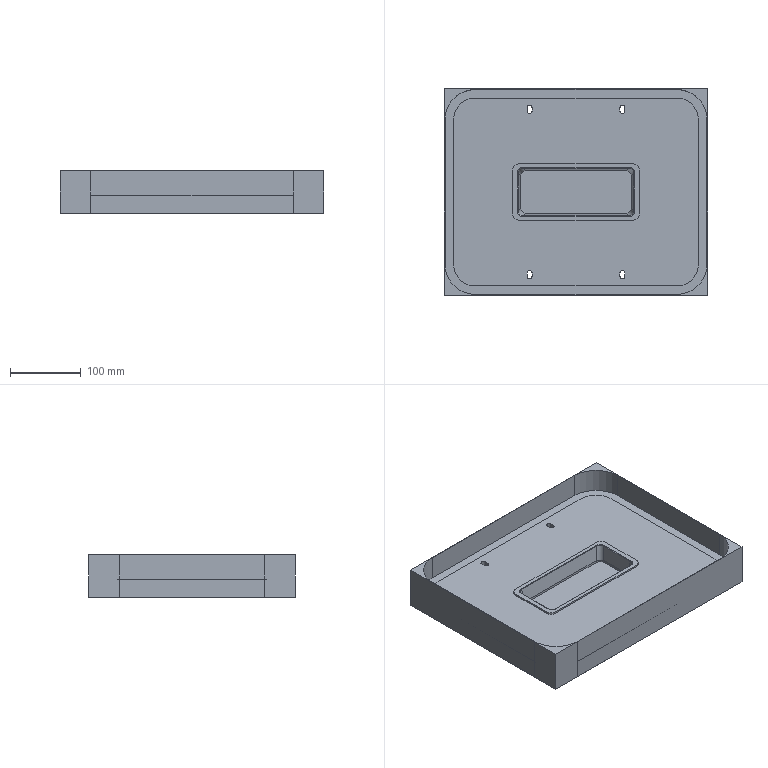NC program | NX | posted with a generic post | part box 371 x 291 x 60.5 mm
Lines 1 to 1445 of 37416:
N10 G17 G21 G94 G90
(CAVITY_MILL , TOOL : D16R0.8)
N12 T00 M6
N14 G53
N16 G17 G0 G90 X-26.999 Y136.323 S8000 M3 M8
N18 G43 Z120.5 H0
N20 Z61.5
N22 G94 G1 X0. Z60.085 F4500.
N24 X142.5
N26 G2 X176.323 Y102.5 R33.823
N28 G1 Y-102.506
N30 G2 X142.5 Y-136.323 R33.823
N32 G1 X-142.5
N34 G2 X-176.323 Y-102.5 R33.823
N36 G1 Y102.5
N38 G2 X-142.5 Y136.323 R33.823
N40 G1 X0.
N42 Y126.243
N44 X142.5
N46 G2 X166.243 Y102.5 R23.743
N48 G1 Y-102.504
N50 G2 X142.5 Y-126.243 R23.743
N52 G1 X-142.5
N54 G2 X-166.243 Y-102.5 R23.743
N56 G1 Y102.5
N58 G2 X-142.5 Y126.243 R23.743
N60 G1 X0.
N62 Y116.163
N64 X142.5
N66 G2 X156.163 Y102.5 R13.663
N68 G1 Y-102.504
N70 G2 X142.5 Y-116.163 R13.663
N72 G1 X-142.5
N74 G2 X-156.163 Y-102.5 R13.663
N76 G1 Y102.5
N78 G2 X-142.5 Y116.163 R13.663
N80 G1 X0.
N82 Y106.083
N84 X142.5
N86 G2 X146.083 Y102.5 R3.583
N88 G1 Y-102.502
N90 G2 X142.5 Y-106.083 R3.583
N92 G1 X-142.5
N94 G2 X-146.083 Y-102.5 R3.583
N96 G1 Y102.5
N98 G2 X-142.5 Y106.083 R3.583
N100 G1 X0.
N102 Y96.003
N104 X136.003
N106 Y-96.003
N108 X-136.003
N110 Y96.003
N112 X0.
N114 Y85.923
N116 X125.923
N118 Y-85.923
N120 X-125.923
N122 Y85.923
N124 X0.
N126 Y75.843
N128 X115.843
N130 Y-75.843
N132 X-115.843
N134 Y75.843
N136 X0.
N138 Y65.763
N140 X105.763
N142 Y-65.763
N144 X-105.763
N146 Y65.763
N148 X0.
N150 Y55.683
N152 X95.683
N154 Y-55.683
N156 X-95.683
N158 Y55.683
N160 X0.
N162 Y45.603
N164 X85.603
N166 Y-45.603
N168 X-85.603
N170 Y45.603
N172 X0.
N174 Y35.523
N176 X75.523
N178 Y-35.523
N180 X-75.523
N182 Y35.523
N184 X0.
N186 Y25.443
N188 X65.443
N190 Y-25.443
N192 X-65.443
N194 Y25.443
N196 X0.
N198 Y15.363
N200 X55.363
N202 Y-15.363
N204 X-55.363
N206 Y15.363
N208 X0.
N210 Y5.283
N212 X45.283
N214 Y-5.283
N216 X-45.283
N218 Y5.283
N220 X0.
N222 G3 X3.2 Y8.483 R3.2
N224 G1 Z61.085
N226 G0 Z63.5
N228 X-26.999 Y136.25
N230 Z61.085
N232 G1 X0. Z59.67
N234 X142.5
N236 G2 X176.25 Y102.506 R33.75
N238 G1 Y-102.506
N240 G2 X142.5 Y-136.25 R33.75
N242 G1 X-142.5
N244 G2 X-176.25 Y-102.5 R33.75
N246 G1 Y102.5
N248 G2 X-142.5 Y136.25 R33.75
N250 G1 X0.
N252 Y126.17
N254 X142.5
N256 G2 X166.17 Y102.504 R23.67
N258 G1 Y-102.504
N260 G2 X142.5 Y-126.17 R23.67
N262 G1 X-142.5
N264 G2 X-166.17 Y-102.5 R23.67
N266 G1 Y102.5
N268 G2 X-142.5 Y126.17 R23.67
N270 G1 X0.
N272 Y116.09
N274 X142.5
N276 G2 X156.09 Y102.502 R13.59
N278 G1 Y-102.504
N280 G2 X142.5 Y-116.09 R13.59
N282 G1 X-142.5
N284 G2 X-156.09 Y-102.5 R13.59
N286 G1 Y102.5
N288 G2 X-142.5 Y116.09 R13.59
N290 G1 X0.
N292 Y106.01
N294 X142.5
N296 G2 X146.01 Y102.501 R3.51
N298 G1 Y-102.502
N300 G2 X142.5 Y-106.01 R3.51
N302 G1 X-142.5
N304 G2 X-146.01 Y-102.5 R3.51
N306 G1 Y102.5
N308 G2 X-142.5 Y106.01 R3.51
N310 G1 X0.
N312 Y95.93
N314 X135.93
N316 Y-95.93
N318 X-135.93
N320 Y95.93
N322 X0.
N324 Y85.85
N326 X125.85
N328 Y-85.85
N330 X-125.85
N332 Y85.85
N334 X0.
N336 Y75.77
N338 X115.77
N340 Y-75.77
N342 X-115.77
N344 Y75.77
N346 X0.
N348 Y65.69
N350 X105.69
N352 Y-65.69
N354 X-105.69
N356 Y65.69
N358 X0.
N360 Y55.61
N362 X95.61
N364 Y-55.61
N366 X-95.61
N368 Y55.61
N370 X0.
N372 Y45.53
N374 X85.53
N376 Y-45.53
N378 X-85.53
N380 Y45.53
N382 X0.
N384 Y35.45
N386 X75.45
N388 Y-35.45
N390 X-75.45
N392 Y35.45
N394 X0.
N396 Y25.37
N398 X65.37
N400 Y-25.37
N402 X-65.37
N404 Y25.37
N406 X0.
N408 Y15.29
N410 X55.29
N412 Y-15.29
N414 X-55.29
N416 Y15.29
N418 X0.
N420 Y5.21
N422 X45.21
N424 Y-5.21
N426 X-45.21
N428 Y5.21
N430 X0.
N432 G3 X3.2 Y8.41 R3.2
N434 G1 Z60.67
N436 G0 Z63.085
N438 X-26.999 Y136.25
N440 Z60.67
N442 G1 X0. Z59.255
N444 X142.5
N446 G2 X176.25 Y102.506 R33.75
N448 G1 Y-102.506
N450 G2 X142.5 Y-136.25 R33.75
N452 G1 X-142.5
N454 G2 X-176.25 Y-102.5 R33.75
N456 G1 Y102.5
N458 G2 X-142.5 Y136.25 R33.75
N460 G1 X0.
N462 Y126.17
N464 X142.5
N466 G2 X166.17 Y102.504 R23.67
N468 G1 Y-102.504
N470 G2 X142.5 Y-126.17 R23.67
N472 G1 X-142.5
N474 G2 X-166.17 Y-102.5 R23.67
N476 G1 Y102.5
N478 G2 X-142.5 Y126.17 R23.67
N480 G1 X0.
N482 Y116.09
N484 X142.5
N486 G2 X156.09 Y102.502 R13.59
N488 G1 Y-102.504
N490 G2 X142.5 Y-116.09 R13.59
N492 G1 X-142.5
N494 G2 X-156.09 Y-102.5 R13.59
N496 G1 Y102.5
N498 G2 X-142.5 Y116.09 R13.59
N500 G1 X0.
N502 Y106.01
N504 X142.5
N506 G2 X146.01 Y102.501 R3.51
N508 G1 Y-102.502
N510 G2 X142.5 Y-106.01 R3.51
N512 G1 X-142.5
N514 G2 X-146.01 Y-102.5 R3.51
N516 G1 Y102.5
N518 G2 X-142.5 Y106.01 R3.51
N520 G1 X0.
N522 Y95.93
N524 X135.93
N526 Y-95.93
N528 X-135.93
N530 Y95.93
N532 X0.
N534 Y85.85
N536 X125.85
N538 Y-85.85
N540 X-125.85
N542 Y85.85
N544 X0.
N546 Y75.77
N548 X115.77
N550 Y-75.77
N552 X-115.77
N554 Y75.77
N556 X0.
N558 Y65.69
N560 X105.69
N562 Y-65.69
N564 X-105.69
N566 Y65.69
N568 X0.
N570 Y55.61
N572 X95.61
N574 Y-55.61
N576 X-95.61
N578 Y55.61
N580 X0.
N582 Y45.53
N584 X85.53
N586 Y-45.53
N588 X-85.53
N590 Y45.53
N592 X0.
N594 Y35.45
N596 X75.45
N598 Y-35.45
N600 X-75.45
N602 Y35.45
N604 X0.
N606 Y25.37
N608 X65.37
N610 Y-25.37
N612 X-65.37
N614 Y25.37
N616 X0.
N618 Y15.29
N620 X55.29
N622 Y-15.29
N624 X-55.29
N626 Y15.29
N628 X0.
N630 Y5.21
N632 X45.21
N634 Y-5.21
N636 X-45.21
N638 Y5.21
N640 X0.
N642 G3 X3.2 Y8.41 R3.2
N644 G1 Z60.255
N646 G0 Z62.67
N648 X-26.999 Y136.25
N650 Z60.255
N652 G1 X0. Z58.84
N654 X142.5
N656 G2 X176.25 Y102.506 R33.75
N658 G1 Y-102.506
N660 G2 X142.5 Y-136.25 R33.75
N662 G1 X-142.5
N664 G2 X-176.25 Y-102.5 R33.75
N666 G1 Y102.5
N668 G2 X-142.5 Y136.25 R33.75
N670 G1 X0.
N672 Y126.17
N674 X142.5
N676 G2 X166.17 Y102.504 R23.67
N678 G1 Y-102.504
N680 G2 X142.5 Y-126.17 R23.67
N682 G1 X-142.5
N684 G2 X-166.17 Y-102.5 R23.67
N686 G1 Y102.5
N688 G2 X-142.5 Y126.17 R23.67
N690 G1 X0.
N692 Y116.09
N694 X142.5
N696 G2 X156.09 Y102.502 R13.59
N698 G1 Y-102.504
N700 G2 X142.5 Y-116.09 R13.59
N702 G1 X-142.5
N704 G2 X-156.09 Y-102.5 R13.59
N706 G1 Y102.5
N708 G2 X-142.5 Y116.09 R13.59
N710 G1 X0.
N712 Y106.01
N714 X142.5
N716 G2 X146.01 Y102.501 R3.51
N718 G1 Y-102.502
N720 G2 X142.5 Y-106.01 R3.51
N722 G1 X-142.5
N724 G2 X-146.01 Y-102.5 R3.51
N726 G1 Y102.5
N728 G2 X-142.5 Y106.01 R3.51
N730 G1 X0.
N732 Y95.93
N734 X135.93
N736 Y-95.93
N738 X-135.93
N740 Y95.93
N742 X0.
N744 Y85.85
N746 X125.85
N748 Y-85.85
N750 X-125.85
N752 Y85.85
N754 X0.
N756 Y75.77
N758 X115.77
N760 Y-75.77
N762 X-115.77
N764 Y75.77
N766 X0.
N768 Y65.69
N770 X105.69
N772 Y-65.69
N774 X-105.69
N776 Y65.69
N778 X0.
N780 Y55.61
N782 X95.61
N784 Y-55.61
N786 X-95.61
N788 Y55.61
N790 X0.
N792 Y45.53
N794 X85.53
N796 Y-45.53
N798 X-85.53
N800 Y45.53
N802 X0.
N804 Y35.45
N806 X75.45
N808 Y-35.45
N810 X-75.45
N812 Y35.45
N814 X0.
N816 Y25.37
N818 X65.37
N820 Y-25.37
N822 X-65.37
N824 Y25.37
N826 X0.
N828 Y15.29
N830 X55.29
N832 Y-15.29
N834 X-55.29
N836 Y15.29
N838 X0.
N840 Y5.21
N842 X45.21
N844 Y-5.21
N846 X-45.21
N848 Y5.21
N850 X0.
N852 G3 X3.2 Y8.41 R3.2
N854 G1 Z59.84
N856 G0 Z62.255
N858 X-26.999 Y136.25
N860 Z59.84
N862 G1 X0. Z58.425
N864 X142.5
N866 G2 X176.25 Y102.506 R33.75
N868 G1 Y-102.506
N870 G2 X142.5 Y-136.25 R33.75
N872 G1 X-142.5
N874 G2 X-176.25 Y-102.5 R33.75
N876 G1 Y102.5
N878 G2 X-142.5 Y136.25 R33.75
N880 G1 X0.
N882 Y126.17
N884 X142.5
N886 G2 X166.17 Y102.504 R23.67
N888 G1 Y-102.504
N890 G2 X142.5 Y-126.17 R23.67
N892 G1 X-142.5
N894 G2 X-166.17 Y-102.5 R23.67
N896 G1 Y102.5
N898 G2 X-142.5 Y126.17 R23.67
N900 G1 X0.
N902 Y116.09
N904 X142.5
N906 G2 X156.09 Y102.502 R13.59
N908 G1 Y-102.504
N910 G2 X142.5 Y-116.09 R13.59
N912 G1 X-142.5
N914 G2 X-156.09 Y-102.5 R13.59
N916 G1 Y102.5
N918 G2 X-142.5 Y116.09 R13.59
N920 G1 X0.
N922 Y106.01
N924 X142.5
N926 G2 X146.01 Y102.501 R3.51
N928 G1 Y-102.502
N930 G2 X142.5 Y-106.01 R3.51
N932 G1 X-142.5
N934 G2 X-146.01 Y-102.5 R3.51
N936 G1 Y102.5
N938 G2 X-142.5 Y106.01 R3.51
N940 G1 X0.
N942 Y95.93
N944 X135.93
N946 Y-95.93
N948 X-135.93
N950 Y95.93
N952 X0.
N954 Y85.85
N956 X125.85
N958 Y-85.85
N960 X-125.85
N962 Y85.85
N964 X0.
N966 Y75.77
N968 X115.77
N970 Y-75.77
N972 X-115.77
N974 Y75.77
N976 X0.
N978 Y65.69
N980 X105.69
N982 Y-65.69
N984 X-105.69
N986 Y65.69
N988 X0.
N990 Y55.61
N992 X95.61
N994 Y-55.61
N996 X-95.61
N998 Y55.61
N1000 X0.
N1002 Y45.53
N1004 X85.53
N1006 Y-45.53
N1008 X-85.53
N1010 Y45.53
N1012 X0.
N1014 Y35.45
N1016 X75.45
N1018 Y-35.45
N1020 X-75.45
N1022 Y35.45
N1024 X0.
N1026 Y25.37
N1028 X65.37
N1030 Y-25.37
N1032 X-65.37
N1034 Y25.37
N1036 X0.
N1038 Y15.29
N1040 X55.29
N1042 Y-15.29
N1044 X-55.29
N1046 Y15.29
N1048 X0.
N1050 Y5.21
N1052 X45.21
N1054 Y-5.21
N1056 X-45.21
N1058 Y5.21
N1060 X0.
N1062 G3 X3.2 Y8.41 R3.2
N1064 G1 Z59.425
N1066 G0 Z61.84
N1068 X-26.999 Y136.25
N1070 Z59.425
N1072 G1 X0. Z58.01
N1074 X142.5
N1076 G2 X176.25 Y102.506 R33.75
N1078 G1 Y-102.506
N1080 G2 X142.5 Y-136.25 R33.75
N1082 G1 X-142.5
N1084 G2 X-176.25 Y-102.5 R33.75
N1086 G1 Y102.5
N1088 G2 X-142.5 Y136.25 R33.75
N1090 G1 X0.
N1092 Y126.17
N1094 X142.5
N1096 G2 X166.17 Y102.504 R23.67
N1098 G1 Y-102.504
N1100 G2 X142.5 Y-126.17 R23.67
N1102 G1 X-142.5
N1104 G2 X-166.17 Y-102.5 R23.67
N1106 G1 Y102.5
N1108 G2 X-142.5 Y126.17 R23.67
N1110 G1 X0.
N1112 Y116.09
N1114 X142.5
N1116 G2 X156.09 Y102.502 R13.59
N1118 G1 Y-102.504
N1120 G2 X142.5 Y-116.09 R13.59
N1122 G1 X-142.5
N1124 G2 X-156.09 Y-102.5 R13.59
N1126 G1 Y102.5
N1128 G2 X-142.5 Y116.09 R13.59
N1130 G1 X0.
N1132 Y106.01
N1134 X142.5
N1136 G2 X146.01 Y102.501 R3.51
N1138 G1 Y-102.502
N1140 G2 X142.5 Y-106.01 R3.51
N1142 G1 X-142.5
N1144 G2 X-146.01 Y-102.5 R3.51
N1146 G1 Y102.5
N1148 G2 X-142.5 Y106.01 R3.51
N1150 G1 X0.
N1152 Y95.93
N1154 X135.93
N1156 Y-95.93
N1158 X-135.93
N1160 Y95.93
N1162 X0.
N1164 Y85.85
N1166 X125.85
N1168 Y-85.85
N1170 X-125.85
N1172 Y85.85
N1174 X0.
N1176 Y75.77
N1178 X115.77
N1180 Y-75.77
N1182 X-115.77
N1184 Y75.77
N1186 X0.
N1188 Y65.69
N1190 X105.69
N1192 Y-65.69
N1194 X-105.69
N1196 Y65.69
N1198 X0.
N1200 Y55.61
N1202 X95.61
N1204 Y-55.61
N1206 X-95.61
N1208 Y55.61
N1210 X0.
N1212 Y45.53
N1214 X85.53
N1216 Y-45.53
N1218 X-85.53
N1220 Y45.53
N1222 X0.
N1224 Y35.45
N1226 X75.45
N1228 Y-35.45
N1230 X-75.45
N1232 Y35.45
N1234 X0.
N1236 Y25.37
N1238 X65.37
N1240 Y-25.37
N1242 X-65.37
N1244 Y25.37
N1246 X0.
N1248 Y15.29
N1250 X55.29
N1252 Y-15.29
N1254 X-55.29
N1256 Y15.29
N1258 X0.
N1260 Y5.21
N1262 X45.21
N1264 Y-5.21
N1266 X-45.21
N1268 Y5.21
N1270 X0.
N1272 G3 X3.2 Y8.41 R3.2
N1274 G1 Z59.01
N1276 G0 Z61.425
N1278 X-26.999 Y136.25
N1280 Z59.01
N1282 G1 X0. Z57.595
N1284 X142.5
N1286 G2 X176.25 Y102.506 R33.75
N1288 G1 Y-102.506
N1290 G2 X142.5 Y-136.25 R33.75
N1292 G1 X-142.5
N1294 G2 X-176.25 Y-102.5 R33.75
N1296 G1 Y102.5
N1298 G2 X-142.5 Y136.25 R33.75
N1300 G1 X0.
N1302 Y126.17
N1304 X142.5
N1306 G2 X166.17 Y102.504 R23.67
N1308 G1 Y-102.504
N1310 G2 X142.5 Y-126.17 R23.67
N1312 G1 X-142.5
N1314 G2 X-166.17 Y-102.5 R23.67
N1316 G1 Y102.5
N1318 G2 X-142.5 Y126.17 R23.67
N1320 G1 X0.
N1322 Y116.09
N1324 X142.5
N1326 G2 X156.09 Y102.502 R13.59
N1328 G1 Y-102.504
N1330 G2 X142.5 Y-116.09 R13.59
N1332 G1 X-142.5
N1334 G2 X-156.09 Y-102.5 R13.59
N1336 G1 Y102.5
N1338 G2 X-142.5 Y116.09 R13.59
N1340 G1 X0.
N1342 Y106.01
N1344 X142.5
N1346 G2 X146.01 Y102.501 R3.51
N1348 G1 Y-102.502
N1350 G2 X142.5 Y-106.01 R3.51
N1352 G1 X-142.5
N1354 G2 X-146.01 Y-102.5 R3.51
N1356 G1 Y102.5
N1358 G2 X-142.5 Y106.01 R3.51
N1360 G1 X0.
N1362 Y95.93
N1364 X135.93
N1366 Y-95.93
N1368 X-135.93
N1370 Y95.93
N1372 X0.
N1374 Y85.85
N1376 X125.85
N1378 Y-85.85
N1380 X-125.85
N1382 Y85.85
N1384 X0.
N1386 Y75.77
N1388 X115.77
N1390 Y-75.77
N1392 X-115.77
N1394 Y75.77
N1396 X0.
N1398 Y65.69
N1400 X105.69
N1402 Y-65.69
N1404 X-105.69
N1406 Y65.69
N1408 X0.
N1410 Y55.61
N1412 X95.61
N1414 Y-55.61
N1416 X-95.61
N1418 Y55.61
N1420 X0.
N1422 Y45.53
N1424 X85.53
N1426 Y-45.53
N1428 X-85.53
N1430 Y45.53
N1432 X0.
N1434 Y35.45
N1436 X75.45
N1438 Y-35.45
N1440 X-75.45
N1442 Y35.45
N1444 X0.
N1446 Y25.37
N1448 X65.37
N1450 Y-25.37
N1452 X-65.37
N1454 Y25.37
N1456 X0.
N1458 Y15.29
N1460 X55.29
N1462 Y-15.29
N1464 X-55.29
N1466 Y15.29
N1468 X0.
N1470 Y5.21
N1472 X45.21
N1474 Y-5.21
N1476 X-45.21
N1478 Y5.21
N1480 X0.
N1482 G3 X3.2 Y8.41 R3.2
N1484 G1 Z58.595
N1486 G0 Z61.01
N1488 X-26.999 Y136.25
N1490 Z58.595
N1492 G1 X0. Z57.181
N1494 X142.5
N1496 G2 X176.25 Y102.506 R33.75
N1498 G1 Y-102.506
N1500 G2 X142.5 Y-136.25 R33.75
N1502 G1 X-142.5
N1504 G2 X-176.25 Y-102.5 R33.75
N1506 G1 Y102.5
N1508 G2 X-142.5 Y136.25 R33.75
N1510 G1 X0.
N1512 Y126.17
N1514 X142.5
N1516 G2 X166.17 Y102.504 R23.67
N1518 G1 Y-102.504
N1520 G2 X142.5 Y-126.17 R23.67
N1522 G1 X-142.5
N1524 G2 X-166.17 Y-102.5 R23.67
N1526 G1 Y102.5
N1528 G2 X-142.5 Y126.17 R23.67
N1530 G1 X0.
N1532 Y116.09
N1534 X142.5
N1536 G2 X156.09 Y102.502 R13.59
N1538 G1 Y-102.504
N1540 G2 X142.5 Y-116.09 R13.59
N1542 G1 X-142.5
N1544 G2 X-156.09 Y-102.5 R13.59
N1546 G1 Y102.5
N1548 G2 X-142.5 Y116.09 R13.59
N1550 G1 X0.
N1552 Y106.01
N1554 X142.5
N1556 G2 X146.01 Y102.501 R3.51
N1558 G1 Y-102.502
N1560 G2 X142.5 Y-106.01 R3.51
N1562 G1 X-142.5
N1564 G2 X-146.01 Y-102.5 R3.51
N1566 G1 Y102.5
N1568 G2 X-142.5 Y106.01 R3.51
N1570 G1 X0.
N1572 Y95.93
N1574 X135.93
N1576 Y-95.93
N1578 X-135.93
N1580 Y95.93
N1582 X0.
N1584 Y85.85
N1586 X125.85
N1588 Y-85.85
N1590 X-125.85
N1592 Y85.85
N1594 X0.
N1596 Y75.77
N1598 X115.77
N1600 Y-75.77
N1602 X-115.77
N1604 Y75.77
N1606 X0.
N1608 Y65.69
N1610 X105.69
N1612 Y-65.69
N1614 X-105.69
N1616 Y65.69
N1618 X0.
N1620 Y55.61
N1622 X95.61
N1624 Y-55.61
N1626 X-95.61
N1628 Y55.61
N1630 X0.
N1632 Y45.53
N1634 X85.53
N1636 Y-45.53
N1638 X-85.53
N1640 Y45.53
N1642 X0.
N1644 Y35.45
N1646 X75.45
N1648 Y-35.45
N1650 X-75.45
N1652 Y35.45
N1654 X0.
N1656 Y25.37
N1658 X65.37
N1660 Y-25.37
N1662 X-65.37
N1664 Y25.37
N1666 X0.
N1668 Y15.29
N1670 X55.29
N1672 Y-15.29
N1674 X-55.29
N1676 Y15.29
N1678 X0.
N1680 Y5.21
N1682 X45.21
N1684 Y-5.21
N1686 X-45.21
N1688 Y5.21
N1690 X0.
N1692 G3 X3.2 Y8.41 R3.2
N1694 G1 Z58.181
N1696 G0 Z60.595
N1698 X-26.999 Y136.25
N1700 Z58.181
N1702 G1 X0. Z56.766
N1704 X142.5
N1706 G2 X176.25 Y102.506 R33.75
N1708 G1 Y-102.506
N1710 G2 X142.5 Y-136.25 R33.75
N1712 G1 X-142.5
N1714 G2 X-176.25 Y-102.5 R33.75
N1716 G1 Y102.5
N1718 G2 X-142.5 Y136.25 R33.75
N1720 G1 X0.
N1722 Y126.17
N1724 X142.5
N1726 G2 X166.17 Y102.504 R23.67
N1728 G1 Y-102.504
N1730 G2 X142.5 Y-126.17 R23.67
N1732 G1 X-142.5
N1734 G2 X-166.17 Y-102.5 R23.67
N1736 G1 Y102.5
N1738 G2 X-142.5 Y126.17 R23.67
N1740 G1 X0.
N1742 Y116.09
N1744 X142.5
N1746 G2 X156.09 Y102.502 R13.59
N1748 G1 Y-102.504
N1750 G2 X142.5 Y-116.09 R13.59
N1752 G1 X-142.5
N1754 G2 X-156.09 Y-102.5 R13.59
N1756 G1 Y102.5
N1758 G2 X-142.5 Y116.09 R13.59
N1760 G1 X0.
N1762 Y106.01
N1764 X142.5
N1766 G2 X146.01 Y102.501 R3.51
N1768 G1 Y-102.502
N1770 G2 X142.5 Y-106.01 R3.51
N1772 G1 X-142.5
N1774 G2 X-146.01 Y-102.5 R3.51
N1776 G1 Y102.5
N1778 G2 X-142.5 Y106.01 R3.51
N1780 G1 X0.
N1782 Y95.93
N1784 X135.93
N1786 Y-95.93
N1788 X-135.93
N1790 Y95.93
N1792 X0.
N1794 Y85.85
N1796 X125.85
N1798 Y-85.85
N1800 X-125.85
N1802 Y85.85
N1804 X0.
N1806 Y75.77
N1808 X115.77
N1810 Y-75.77
N1812 X-115.77
N1814 Y75.77
N1816 X0.
N1818 Y65.69
N1820 X105.69
N1822 Y-65.69
N1824 X-105.69
N1826 Y65.69
N1828 X0.
N1830 Y55.61
N1832 X95.61
N1834 Y-55.61
N1836 X-95.61
N1838 Y55.61
N1840 X0.
N1842 Y45.53
N1844 X85.53
N1846 Y-45.53
N1848 X-85.53
N1850 Y45.53
N1852 X0.
N1854 Y35.45
N1856 X75.45
N1858 Y-35.45
N1860 X-75.45
N1862 Y35.45
N1864 X0.
N1866 Y25.37
N1868 X65.37
N1870 Y-25.37
N1872 X-65.37
N1874 Y25.37
N1876 X0.
N1878 Y15.29
N1880 X55.29
N1882 Y-15.29
N1884 X-55.29
N1886 Y15.29
N1888 X0.
N1890 Y5.21
N1892 X45.21
N1894 Y-5.21
N1896 X-45.21
N1898 Y5.21
N1900 X0.
N1902 G3 X3.2 Y8.41 R3.2
N1904 G1 Z57.766
N1906 G0 Z60.181
N1908 X-26.999 Y136.25
N1910 Z57.766
N1912 G1 X0. Z56.351
N1914 X142.5
N1916 G2 X176.25 Y102.506 R33.75
N1918 G1 Y-102.506
N1920 G2 X142.5 Y-136.25 R33.75
N1922 G1 X-142.5
N1924 G2 X-176.25 Y-102.5 R33.75
N1926 G1 Y102.5
N1928 G2 X-142.5 Y136.25 R33.75
N1930 G1 X0.
N1932 Y126.17
N1934 X142.5
N1936 G2 X166.17 Y102.504 R23.67
N1938 G1 Y-102.504
N1940 G2 X142.5 Y-126.17 R23.67
N1942 G1 X-142.5
N1944 G2 X-166.17 Y-102.5 R23.67
N1946 G1 Y102.5
N1948 G2 X-142.5 Y126.17 R23.67
N1950 G1 X0.
N1952 Y116.09
N1954 X142.5
N1956 G2 X156.09 Y102.502 R13.59
N1958 G1 Y-102.504
N1960 G2 X142.5 Y-116.09 R13.59
N1962 G1 X-142.5
N1964 G2 X-156.09 Y-102.5 R13.59
N1966 G1 Y102.5
N1968 G2 X-142.5 Y116.09 R13.59
N1970 G1 X0.
N1972 Y106.01
N1974 X142.5
N1976 G2 X146.01 Y102.501 R3.51
N1978 G1 Y-102.502
N1980 G2 X142.5 Y-106.01 R3.51
N1982 G1 X-142.5
N1984 G2 X-146.01 Y-102.5 R3.51
N1986 G1 Y102.5
N1988 G2 X-142.5 Y106.01 R3.51
N1990 G1 X0.
N1992 Y95.93
N1994 X135.93
N1996 Y-95.93
N1998 X-135.93
N2000 Y95.93
N2002 X0.
N2004 Y85.85
N2006 X125.85
N2008 Y-85.85
N2010 X-125.85
N2012 Y85.85
N2014 X0.
N2016 Y75.77
N2018 X115.77
N2020 Y-75.77
N2022 X-115.77
N2024 Y75.77
N2026 X0.
N2028 Y65.69
N2030 X105.69
N2032 Y-65.69
N2034 X-105.69
N2036 Y65.69
N2038 X0.
N2040 Y55.61
N2042 X95.61
N2044 Y-55.61
N2046 X-95.61
N2048 Y55.61
N2050 X0.
N2052 Y45.53
N2054 X85.53
N2056 Y-45.53
N2058 X-85.53
N2060 Y45.53
N2062 X0.
N2064 Y35.45
N2066 X75.45
N2068 Y-35.45
N2070 X-75.45
N2072 Y35.45
N2074 X0.
N2076 Y25.37
N2078 X65.37
N2080 Y-25.37
N2082 X-65.37
N2084 Y25.37
N2086 X0.
N2088 Y15.29
N2090 X55.29
N2092 Y-15.29
N2094 X-55.29
N2096 Y15.29
N2098 X0.
N2100 Y5.21
N2102 X45.21
N2104 Y-5.21
N2106 X-45.21
N2108 Y5.21
N2110 X0.
N2112 G3 X3.2 Y8.41 R3.2
N2114 G1 Z57.351
N2116 G0 Z59.766
N2118 X-26.999 Y136.25
N2120 Z57.351
N2122 G1 X0. Z55.936
N2124 X142.5
N2126 G2 X176.25 Y102.506 R33.75
N2128 G1 Y-102.506
N2130 G2 X142.5 Y-136.25 R33.75
N2132 G1 X-142.5
N2134 G2 X-176.25 Y-102.5 R33.75
N2136 G1 Y102.5
N2138 G2 X-142.5 Y136.25 R33.75
N2140 G1 X0.
N2142 Y126.17
N2144 X142.5
N2146 G2 X166.17 Y102.504 R23.67
N2148 G1 Y-102.504
N2150 G2 X142.5 Y-126.17 R23.67
N2152 G1 X-142.5
N2154 G2 X-166.17 Y-102.5 R23.67
N2156 G1 Y102.5
N2158 G2 X-142.5 Y126.17 R23.67
N2160 G1 X0.
N2162 Y116.09
N2164 X142.5
N2166 G2 X156.09 Y102.502 R13.59
N2168 G1 Y-102.504
N2170 G2 X142.5 Y-116.09 R13.59
N2172 G1 X-142.5
N2174 G2 X-156.09 Y-102.5 R13.59
N2176 G1 Y102.5
N2178 G2 X-142.5 Y116.09 R13.59
N2180 G1 X0.
N2182 Y106.01
N2184 X142.5
N2186 G2 X146.01 Y102.501 R3.51
N2188 G1 Y-102.502
N2190 G2 X142.5 Y-106.01 R3.51
N2192 G1 X-142.5
N2194 G2 X-146.01 Y-102.5 R3.51
N2196 G1 Y102.5
N2198 G2 X-142.5 Y106.01 R3.51
N2200 G1 X0.
N2202 Y95.93
N2204 X135.93
N2206 Y-95.93
N2208 X-135.93
N2210 Y95.93
N2212 X0.
N2214 Y85.85
N2216 X125.85
N2218 Y-85.85
N2220 X-125.85
N2222 Y85.85
N2224 X0.
N2226 Y75.77
N2228 X115.77
N2230 Y-75.77
N2232 X-115.77
N2234 Y75.77
N2236 X0.
N2238 Y65.69
N2240 X105.69
N2242 Y-65.69
N2244 X-105.69
N2246 Y65.69
N2248 X0.
N2250 Y55.61
N2252 X95.61
N2254 Y-55.61
N2256 X-95.61
N2258 Y55.61
N2260 X0.
N2262 Y45.53
N2264 X85.53
N2266 Y-45.53
N2268 X-85.53
N2270 Y45.53
N2272 X0.
N2274 Y35.45
N2276 X75.45
N2278 Y-35.45
N2280 X-75.45
N2282 Y35.45
N2284 X0.
N2286 Y25.37
N2288 X65.37
N2290 Y-25.37
N2292 X-65.37
N2294 Y25.37
N2296 X0.
N2298 Y15.29
N2300 X55.29
N2302 Y-15.29
N2304 X-55.29
N2306 Y15.29
N2308 X0.
N2310 Y5.21
N2312 X45.21
N2314 Y-5.21
N2316 X-45.21
N2318 Y5.21
N2320 X0.
N2322 G3 X3.2 Y8.41 R3.2
N2324 G1 Z56.936
N2326 G0 Z59.351
N2328 X-26.999 Y136.25
N2330 Z56.936
N2332 G1 X0. Z55.521
N2334 X142.5
N2336 G2 X176.25 Y102.506 R33.75
N2338 G1 Y-102.506
N2340 G2 X142.5 Y-136.25 R33.75
N2342 G1 X-142.5
N2344 G2 X-176.25 Y-102.5 R33.75
N2346 G1 Y102.5
N2348 G2 X-142.5 Y136.25 R33.75
N2350 G1 X0.
N2352 Y126.17
N2354 X142.5
N2356 G2 X166.17 Y102.504 R23.67
N2358 G1 Y-102.504
N2360 G2 X142.5 Y-126.17 R23.67
N2362 G1 X-142.5
N2364 G2 X-166.17 Y-102.5 R23.67
N2366 G1 Y102.5
N2368 G2 X-142.5 Y126.17 R23.67
N2370 G1 X0.
N2372 Y116.09
N2374 X142.5
N2376 G2 X156.09 Y102.502 R13.59
N2378 G1 Y-102.504
N2380 G2 X142.5 Y-116.09 R13.59
N2382 G1 X-142.5
N2384 G2 X-156.09 Y-102.5 R13.59
N2386 G1 Y102.5
N2388 G2 X-142.5 Y116.09 R13.59
N2390 G1 X0.
N2392 Y106.01
N2394 X142.5
N2396 G2 X146.01 Y102.501 R3.51
N2398 G1 Y-102.502
N2400 G2 X142.5 Y-106.01 R3.51
N2402 G1 X-142.5
N2404 G2 X-146.01 Y-102.5 R3.51
N2406 G1 Y102.5
N2408 G2 X-142.5 Y106.01 R3.51
N2410 G1 X0.
N2412 Y95.93
N2414 X135.93
N2416 Y-95.93
N2418 X-135.93
N2420 Y95.93
N2422 X0.
N2424 Y85.85
N2426 X125.85
N2428 Y-85.85
N2430 X-125.85
N2432 Y85.85
N2434 X0.
N2436 Y75.77
N2438 X115.77
N2440 Y-75.77
N2442 X-115.77
N2444 Y75.77
N2446 X0.
N2448 Y65.69
N2450 X105.69
N2452 Y-65.69
N2454 X-105.69
N2456 Y65.69
N2458 X0.
N2460 Y55.61
N2462 X95.61
N2464 Y-55.61
N2466 X-95.61
N2468 Y55.61
N2470 X0.
N2472 Y45.53
N2474 X85.53
N2476 Y-45.53
N2478 X-85.53
N2480 Y45.53
N2482 X0.
N2484 Y35.45
N2486 X75.45
N2488 Y-35.45
N2490 X-75.45
N2492 Y35.45
N2494 X0.
N2496 Y25.37
N2498 X65.37
N2500 Y-25.37
N2502 X-65.37
N2504 Y25.37
N2506 X0.
N2508 Y15.29
N2510 X55.29
N2512 Y-15.29
N2514 X-55.29
N2516 Y15.29
N2518 X0.
N2520 Y5.21
N2522 X45.21
N2524 Y-5.21
N2526 X-45.21
N2528 Y5.21
N2530 X0.
N2532 G3 X3.2 Y8.41 R3.2
N2534 G1 Z56.521
N2536 G0 Z58.936
N2538 X-26.999 Y136.25
N2540 Z56.521
N2542 G1 X0. Z55.106
N2544 X142.5
N2546 G2 X176.25 Y102.506 R33.75
N2548 G1 Y-102.506
N2550 G2 X142.5 Y-136.25 R33.75
N2552 G1 X-142.5
N2554 G2 X-176.25 Y-102.5 R33.75
N2556 G1 Y102.5
N2558 G2 X-142.5 Y136.25 R33.75
N2560 G1 X0.
N2562 Y126.17
N2564 X142.5
N2566 G2 X166.17 Y102.504 R23.67
N2568 G1 Y-102.504
N2570 G2 X142.5 Y-126.17 R23.67
N2572 G1 X-142.5
N2574 G2 X-166.17 Y-102.5 R23.67
N2576 G1 Y102.5
N2578 G2 X-142.5 Y126.17 R23.67
N2580 G1 X0.
N2582 Y116.09
N2584 X142.5
N2586 G2 X156.09 Y102.502 R13.59
N2588 G1 Y-102.504
N2590 G2 X142.5 Y-116.09 R13.59
N2592 G1 X-142.5
N2594 G2 X-156.09 Y-102.5 R13.59
N2596 G1 Y102.5
N2598 G2 X-142.5 Y116.09 R13.59
N2600 G1 X0.
N2602 Y106.01
N2604 X142.5
N2606 G2 X146.01 Y102.501 R3.51
N2608 G1 Y-102.502
N2610 G2 X142.5 Y-106.01 R3.51
N2612 G1 X-142.5
N2614 G2 X-146.01 Y-102.5 R3.51
N2616 G1 Y102.5
N2618 G2 X-142.5 Y106.01 R3.51
N2620 G1 X0.
N2622 Y95.93
N2624 X135.93
N2626 Y-95.93
N2628 X-135.93
N2630 Y95.93
N2632 X0.
N2634 Y85.85
N2636 X125.85
N2638 Y-85.85
N2640 X-125.85
N2642 Y85.85
N2644 X0.
N2646 Y75.77
N2648 X115.77
N2650 Y-75.77
N2652 X-115.77
N2654 Y75.77
N2656 X0.
N2658 Y65.69
N2660 X105.69
N2662 Y-65.69
N2664 X-105.69
N2666 Y65.69
N2668 X0.
N2670 Y55.61
N2672 X95.61
N2674 Y-55.61
N2676 X-95.61
N2678 Y55.61
N2680 X0.
N2682 Y45.53
N2684 X85.53
N2686 Y-45.53
N2688 X-85.53
N2690 Y45.53
N2692 X0.
N2694 Y35.45
N2696 X75.45
N2698 Y-35.45
N2700 X-75.45
N2702 Y35.45
N2704 X0.
N2706 Y25.37
N2708 X65.37
N2710 Y-25.37
N2712 X-65.37
N2714 Y25.37
N2716 X0.
N2718 Y15.29
N2720 X55.29
N2722 Y-15.29
N2724 X-55.29
N2726 Y15.29
N2728 X0.
N2730 Y5.21
N2732 X45.21
N2734 Y-5.21
N2736 X-45.21
N2738 Y5.21
N2740 X0.
N2742 G3 X3.2 Y8.41 R3.2
N2744 G1 Z56.106
N2746 G0 Z58.521
N2748 X-26.999 Y136.25
N2750 Z56.106
N2752 G1 X0. Z54.691
N2754 X142.5
N2756 G2 X176.25 Y102.506 R33.75
N2758 G1 Y-102.506
N2760 G2 X142.5 Y-136.25 R33.75
N2762 G1 X-142.5
N2764 G2 X-176.25 Y-102.5 R33.75
N2766 G1 Y102.5
N2768 G2 X-142.5 Y136.25 R33.75
N2770 G1 X0.
N2772 Y126.17
N2774 X142.5
N2776 G2 X166.17 Y102.504 R23.67
N2778 G1 Y-102.504
N2780 G2 X142.5 Y-126.17 R23.67
N2782 G1 X-142.5
N2784 G2 X-166.17 Y-102.5 R23.67
N2786 G1 Y102.5
N2788 G2 X-142.5 Y126.17 R23.67
N2790 G1 X0.
N2792 Y116.09
N2794 X142.5
N2796 G2 X156.09 Y102.502 R13.59
N2798 G1 Y-102.504
N2800 G2 X142.5 Y-116.09 R13.59
N2802 G1 X-142.5
N2804 G2 X-156.09 Y-102.5 R13.59
N2806 G1 Y102.5
N2808 G2 X-142.5 Y116.09 R13.59
N2810 G1 X0.
N2812 Y106.01
N2814 X142.5
N2816 G2 X146.01 Y102.501 R3.51
N2818 G1 Y-102.502
N2820 G2 X142.5 Y-106.01 R3.51
N2822 G1 X-142.5
N2824 G2 X-146.01 Y-102.5 R3.51
N2826 G1 Y102.5
N2828 G2 X-142.5 Y106.01 R3.51
N2830 G1 X0.
N2832 Y95.93
N2834 X135.93
N2836 Y-95.93
N2838 X-135.93
N2840 Y95.93
N2842 X0.
N2844 Y85.85
N2846 X125.85
N2848 Y-85.85
N2850 X-125.85
N2852 Y85.85
N2854 X0.
N2856 Y75.77
N2858 X115.77
N2860 Y-75.77
N2862 X-115.77
N2864 Y75.77
N2866 X0.
N2868 Y65.69
N2870 X105.69
N2872 Y-65.69
N2874 X-105.69
N2876 Y65.69
N2878 X0.
N2880 Y55.61
N2882 X95.61
N2884 Y-55.61
N2886 X-95.61
N2888 Y55.61